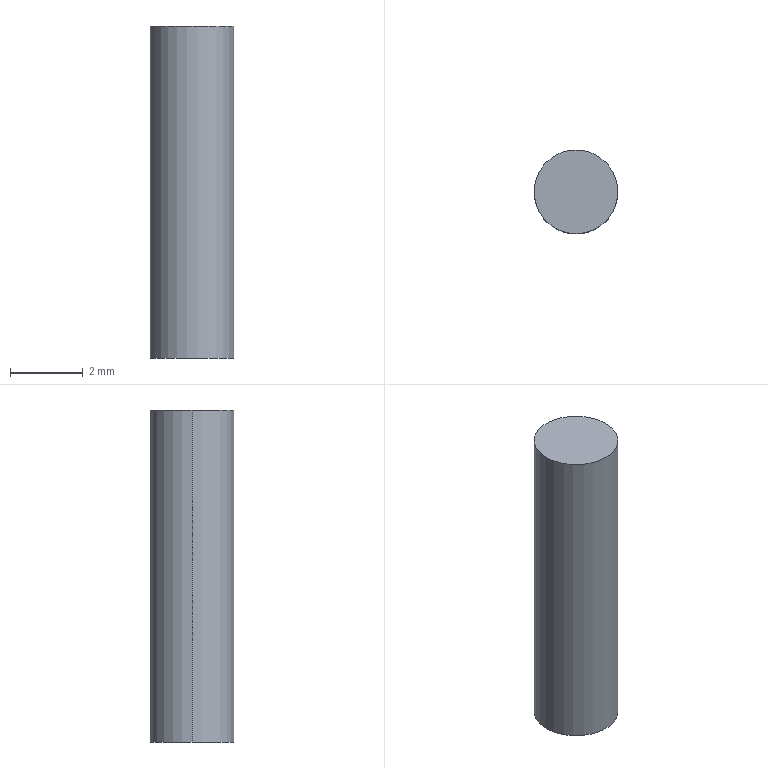Part | SolidWorks | features Extrusion 1 | 1 solid | 4 faces | box 2.3 x 2.3 x 9.1 mm | volume 37.808 mm3 | cylinder 2 | plane 2 | commonest cylinder face diameters 2.3 x2
STEP:
#1=CARTESIAN_POINT('',(1.15,0.,9.1));
#2=VERTEX_POINT('',#1);
#3=CARTESIAN_POINT('',(-1.15,0.,9.1));
#4=VERTEX_POINT('',#3);
#5=CARTESIAN_POINT('',(0.,0.,9.1));
#6=DIRECTION('',(0.,0.,1.));
#7=DIRECTION('',(1.,0.,0.));
#8=AXIS2_PLACEMENT_3D('',#5,#6,#7);
#9=CIRCLE('',#8,1.15);
#10=EDGE_CURVE('',#2,#4,#9,.T.);
#11=ORIENTED_EDGE('',*,*,#10,.F.);
#12=CARTESIAN_POINT('',(1.15,0.,0.));
#13=VERTEX_POINT('',#12);
#14=CARTESIAN_POINT('',(1.15,0.,9.1));
#15=DIRECTION('',(0.,0.,-1.));
#16=VECTOR('',#15,1000.);
#17=LINE('',#14,#16);
#18=EDGE_CURVE('',#2,#13,#17,.T.);
#19=ORIENTED_EDGE('',*,*,#18,.T.);
#20=CARTESIAN_POINT('',(-1.15,0.,0.));
#21=VERTEX_POINT('',#20);
#22=CARTESIAN_POINT('',(0.,0.,0.));
#23=DIRECTION('',(0.,0.,1.));
#24=DIRECTION('',(1.,0.,0.));
#25=AXIS2_PLACEMENT_3D('',#22,#23,#24);
#26=CIRCLE('',#25,1.15);
#27=EDGE_CURVE('',#13,#21,#26,.T.);
#28=ORIENTED_EDGE('',*,*,#27,.T.);
#29=CARTESIAN_POINT('',(-1.15,0.,9.1));
#30=DIRECTION('',(0.,0.,-1.));
#31=VECTOR('',#30,1000.);
#32=LINE('',#29,#31);
#33=EDGE_CURVE('',#4,#21,#32,.T.);
#34=ORIENTED_EDGE('',*,*,#33,.F.);
#35=EDGE_LOOP('',(#11,#19,#28,#34));
#36=FACE_OUTER_BOUND('',#35,.T.);
#37=CARTESIAN_POINT('',(0.,0.,9.1));
#38=DIRECTION('',(0.,0.,-1.));
#39=DIRECTION('',(-1.,0.,0.));
#40=AXIS2_PLACEMENT_3D('',#37,#38,#39);
#41=CYLINDRICAL_SURFACE('',#40,1.15);
#42=ADVANCED_FACE('',(#36),#41,.T.);
#43=ORIENTED_EDGE('',*,*,#18,.F.);
#44=CARTESIAN_POINT('',(0.,0.,9.1));
#45=DIRECTION('',(0.,0.,1.));
#46=DIRECTION('',(1.,0.,0.));
#47=AXIS2_PLACEMENT_3D('',#44,#45,#46);
#48=CIRCLE('',#47,1.15);
#49=EDGE_CURVE('',#4,#2,#48,.T.);
#50=ORIENTED_EDGE('',*,*,#49,.F.);
#51=ORIENTED_EDGE('',*,*,#33,.T.);
#52=CARTESIAN_POINT('',(0.,0.,0.));
#53=DIRECTION('',(0.,0.,1.));
#54=DIRECTION('',(1.,0.,0.));
#55=AXIS2_PLACEMENT_3D('',#52,#53,#54);
#56=CIRCLE('',#55,1.15);
#57=EDGE_CURVE('',#21,#13,#56,.T.);
#58=ORIENTED_EDGE('',*,*,#57,.T.);
#59=EDGE_LOOP('',(#43,#50,#51,#58));
#60=FACE_OUTER_BOUND('',#59,.T.);
#61=CARTESIAN_POINT('',(0.,0.,9.1));
#62=DIRECTION('',(0.,0.,-1.));
#63=DIRECTION('',(-1.,0.,0.));
#64=AXIS2_PLACEMENT_3D('',#61,#62,#63);
#65=CYLINDRICAL_SURFACE('',#64,1.15);
#66=ADVANCED_FACE('',(#60),#65,.T.);
#67=ORIENTED_EDGE('',*,*,#49,.T.);
#68=ORIENTED_EDGE('',*,*,#10,.T.);
#69=EDGE_LOOP('',(#67,#68));
#70=FACE_OUTER_BOUND('',#69,.T.);
#71=CARTESIAN_POINT('',(0.,0.,9.1));
#72=DIRECTION('',(0.,0.,1.));
#73=DIRECTION('',(1.,0.,0.));
#74=AXIS2_PLACEMENT_3D('',#71,#72,#73);
#75=PLANE('',#74);
#76=ADVANCED_FACE('',(#70),#75,.T.);
#77=ORIENTED_EDGE('',*,*,#57,.F.);
#78=ORIENTED_EDGE('',*,*,#27,.F.);
#79=EDGE_LOOP('',(#77,#78));
#80=FACE_OUTER_BOUND('',#79,.T.);
#81=CARTESIAN_POINT('',(0.,0.,0.));
#82=DIRECTION('',(0.,0.,1.));
#83=DIRECTION('',(1.,0.,0.));
#84=AXIS2_PLACEMENT_3D('',#81,#82,#83);
#85=PLANE('',#84);
#86=ADVANCED_FACE('',(#80),#85,.F.);
#87=CLOSED_SHELL('',(#42,#66,#76,#86));
#88=MANIFOLD_SOLID_BREP('',#87);
#89=CARTESIAN_POINT('',(0.,0.,0.));
#90=DIRECTION('',(0.,0.,1.));
#91=DIRECTION('',(1.,0.,0.));
#92=AXIS2_PLACEMENT_3D('',#89,#90,#91);
#93=(LENGTH_UNIT()NAMED_UNIT(*)SI_UNIT(.MILLI.,.METRE.));
#94=UNCERTAINTY_MEASURE_WITH_UNIT(LENGTH_MEASURE(0.00001),#93,'','');
#95=(NAMED_UNIT(*)PLANE_ANGLE_UNIT()SI_UNIT($,.RADIAN.));
#96=(NAMED_UNIT(*)SI_UNIT($,.STERADIAN.)SOLID_ANGLE_UNIT());
#97=(GEOMETRIC_REPRESENTATION_CONTEXT(3)GLOBAL_UNCERTAINTY_ASSIGNED_CONTEXT((#94))GLOBAL_UNIT_ASSIGNED_CONTEXT((#93,#95,#96))REPRESENTATION_CONTEXT('',''));
#98=ADVANCED_BREP_SHAPE_REPRESENTATION('',(#88,#92),#97);